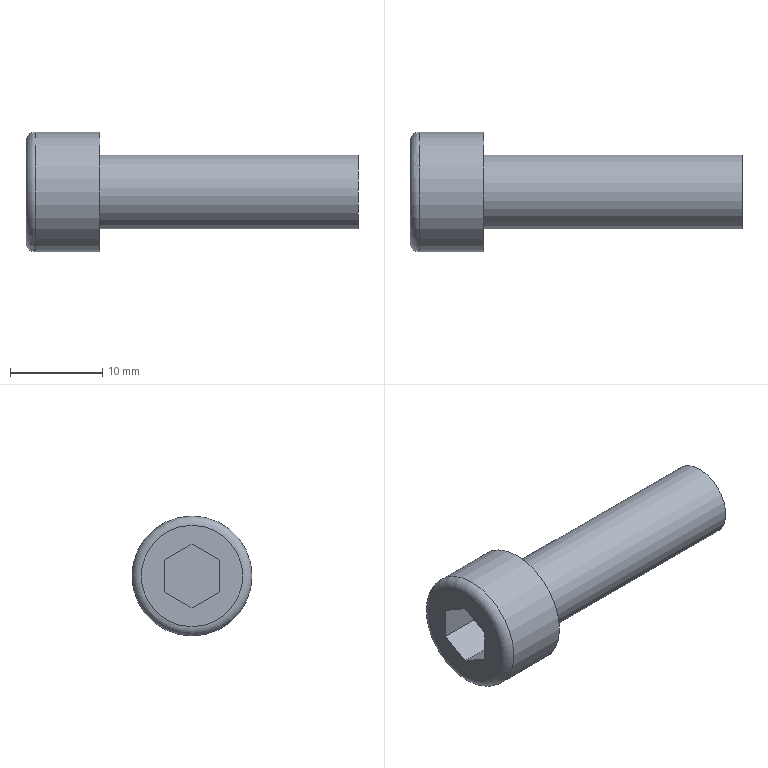Part | STEP file | Tube necking machine_id606_x_t | 1 solid | 13 faces | box 36 x 13 x 13 mm | volume 2296 mm3 | plane 10 | cylinder 2 | torus 1 | commonest cylinder face diameters 8 x1 13 x1
STEP:
#1=CARTESIAN_POINT('',(0.,0.,0.));
#2=DIRECTION('',(0.,0.,1.));
#3=DIRECTION('',(1.,0.,0.));
#4=AXIS2_PLACEMENT_3D('',#1,#2,#3);
#5=CARTESIAN_POINT('',(367.5,70.,164.5));
#6=VERTEX_POINT('',#5);
#7=CARTESIAN_POINT('',(367.5,70.,170.));
#8=DIRECTION('',(-1.,0.,0.));
#9=DIRECTION('',(0.,0.,-1.));
#10=AXIS2_PLACEMENT_3D('',#7,#8,#9);
#11=CIRCLE('',#10,5.5);
#12=CARTESIAN_POINT('',(367.5,70.,176.5));
#13=DIRECTION('',(1.,0.,0.));
#14=DIRECTION('',(0.,0.,-1.));
#15=AXIS2_PLACEMENT_3D('',#12,#13,#14);
#16=PLANE('',#15);
#17=CARTESIAN_POINT('',(12.,0.));
#18=CARTESIAN_POINT('',(12.,-9.526));
#19=CARTESIAN_POINT('',(3.75,-4.763));
#20=CARTESIAN_POINT('',(-4.5,0.));
#21=CARTESIAN_POINT('',(3.75,4.763));
#22=CARTESIAN_POINT('',(12.,9.526));
#23=CARTESIAN_POINT('',(12.,0.));
#24=(BOUNDED_CURVE()B_SPLINE_CURVE(2,(#17,#18,#19,#20,#21,#22,#23),.UNSPECIFIED.,.T.,.F.)B_SPLINE_CURVE_WITH_KNOTS((1,2,2,2,2,1),(-2.094,0.,2.094,4.189,6.283,8.378),.UNSPECIFIED.)CURVE()GEOMETRIC_REPRESENTATION_ITEM()RATIONAL_B_SPLINE_CURVE((1.,0.5,1.,0.5,1.,0.5,1.))REPRESENTATION_ITEM(''));
#25=(GEOMETRIC_REPRESENTATION_CONTEXT(2)PARAMETRIC_REPRESENTATION_CONTEXT()REPRESENTATION_CONTEXT('',''));
#26=DEFINITIONAL_REPRESENTATION('',(#24),#25);
#27=PCURVE('',#16,#26);
#28=CARTESIAN_POINT('',(368.5,70.,170.));
#29=DIRECTION('',(1.,0.,0.));
#30=DIRECTION('',(0.,0.,-1.));
#31=AXIS2_PLACEMENT_3D('',#28,#29,#30);
#32=TOROIDAL_SURFACE('',#31,5.5,1.);
#33=CARTESIAN_POINT('',(6.283,4.712));
#34=DIRECTION('',(-1.,0.));
#35=VECTOR('',#34,1.);
#36=LINE('',#33,#35);
#37=(GEOMETRIC_REPRESENTATION_CONTEXT(2)PARAMETRIC_REPRESENTATION_CONTEXT()REPRESENTATION_CONTEXT('',''));
#38=DEFINITIONAL_REPRESENTATION('',(#36),#37);
#39=PCURVE('',#32,#38);
#40=SURFACE_CURVE('',#11,(#27,#39),.PCURVE_S1.);
#41=EDGE_CURVE('',#6,#6,#40,.T.);
#42=ORIENTED_EDGE('',*,*,#41,.T.);
#43=EDGE_LOOP('',(#42));
#44=FACE_BOUND('',#43,.T.);
#45=CARTESIAN_POINT('',(367.5,73.,168.268));
#46=VERTEX_POINT('',#45);
#47=CARTESIAN_POINT('',(367.5,73.,171.732));
#48=VERTEX_POINT('',#47);
#49=CARTESIAN_POINT('',(367.5,73.,168.268));
#50=DIRECTION('',(0.,0.,1.));
#51=VECTOR('',#50,1.);
#52=LINE('',#49,#51);
#53=CARTESIAN_POINT('',(8.232,3.));
#54=DIRECTION('',(-1.,0.));
#55=VECTOR('',#54,1.);
#56=LINE('',#53,#55);
#57=(GEOMETRIC_REPRESENTATION_CONTEXT(2)PARAMETRIC_REPRESENTATION_CONTEXT()REPRESENTATION_CONTEXT('',''));
#58=DEFINITIONAL_REPRESENTATION('',(#56),#57);
#59=PCURVE('',#16,#58);
#60=CARTESIAN_POINT('',(372.78,73.,168.268));
#61=DIRECTION('',(0.,-1.,0.));
#62=DIRECTION('',(0.,0.,1.));
#63=AXIS2_PLACEMENT_3D('',#60,#61,#62);
#64=PLANE('',#63);
#65=CARTESIAN_POINT('',(0.,5.28));
#66=DIRECTION('',(1.,0.));
#67=VECTOR('',#66,1.);
#68=LINE('',#65,#67);
#69=(GEOMETRIC_REPRESENTATION_CONTEXT(2)PARAMETRIC_REPRESENTATION_CONTEXT()REPRESENTATION_CONTEXT('',''));
#70=DEFINITIONAL_REPRESENTATION('',(#68),#69);
#71=PCURVE('',#64,#70);
#72=SURFACE_CURVE('',#52,(#59,#71),.PCURVE_S1.);
#73=EDGE_CURVE('',#46,#48,#72,.T.);
#74=ORIENTED_EDGE('',*,*,#73,.T.);
#75=CARTESIAN_POINT('',(367.5,70.,173.464));
#76=VERTEX_POINT('',#75);
#77=CARTESIAN_POINT('',(367.5,73.,171.732));
#78=DIRECTION('',(0.,-0.866,0.5));
#79=VECTOR('',#78,1.);
#80=LINE('',#77,#79);
#81=CARTESIAN_POINT('',(4.768,3.));
#82=DIRECTION('',(-0.5,-0.866));
#83=VECTOR('',#82,1.);
#84=LINE('',#81,#83);
#85=(GEOMETRIC_REPRESENTATION_CONTEXT(2)PARAMETRIC_REPRESENTATION_CONTEXT()REPRESENTATION_CONTEXT('',''));
#86=DEFINITIONAL_REPRESENTATION('',(#84),#85);
#87=PCURVE('',#16,#86);
#88=CARTESIAN_POINT('',(372.78,73.,171.732));
#89=DIRECTION('',(0.,-0.5,-0.866));
#90=DIRECTION('',(0.,-0.866,0.5));
#91=AXIS2_PLACEMENT_3D('',#88,#89,#90);
#92=PLANE('',#91);
#93=CARTESIAN_POINT('',(0.,5.28));
#94=DIRECTION('',(1.,0.));
#95=VECTOR('',#94,1.);
#96=LINE('',#93,#95);
#97=(GEOMETRIC_REPRESENTATION_CONTEXT(2)PARAMETRIC_REPRESENTATION_CONTEXT()REPRESENTATION_CONTEXT('',''));
#98=DEFINITIONAL_REPRESENTATION('',(#96),#97);
#99=PCURVE('',#92,#98);
#100=SURFACE_CURVE('',#80,(#87,#99),.PCURVE_S1.);
#101=EDGE_CURVE('',#48,#76,#100,.T.);
#102=ORIENTED_EDGE('',*,*,#101,.T.);
#103=CARTESIAN_POINT('',(367.5,67.,171.732));
#104=VERTEX_POINT('',#103);
#105=CARTESIAN_POINT('',(367.5,70.,173.464));
#106=DIRECTION('',(0.,-0.866,-0.5));
#107=VECTOR('',#106,1.);
#108=LINE('',#105,#107);
#109=CARTESIAN_POINT('',(3.036,0.));
#110=DIRECTION('',(0.5,-0.866));
#111=VECTOR('',#110,1.);
#112=LINE('',#109,#111);
#113=(GEOMETRIC_REPRESENTATION_CONTEXT(2)PARAMETRIC_REPRESENTATION_CONTEXT()REPRESENTATION_CONTEXT('',''));
#114=DEFINITIONAL_REPRESENTATION('',(#112),#113);
#115=PCURVE('',#16,#114);
#116=CARTESIAN_POINT('',(372.78,70.,173.464));
#117=DIRECTION('',(0.,0.5,-0.866));
#118=DIRECTION('',(0.,-0.866,-0.5));
#119=AXIS2_PLACEMENT_3D('',#116,#117,#118);
#120=PLANE('',#119);
#121=CARTESIAN_POINT('',(0.,5.28));
#122=DIRECTION('',(1.,0.));
#123=VECTOR('',#122,1.);
#124=LINE('',#121,#123);
#125=(GEOMETRIC_REPRESENTATION_CONTEXT(2)PARAMETRIC_REPRESENTATION_CONTEXT()REPRESENTATION_CONTEXT('',''));
#126=DEFINITIONAL_REPRESENTATION('',(#124),#125);
#127=PCURVE('',#120,#126);
#128=SURFACE_CURVE('',#108,(#115,#127),.PCURVE_S1.);
#129=EDGE_CURVE('',#76,#104,#128,.T.);
#130=ORIENTED_EDGE('',*,*,#129,.T.);
#131=CARTESIAN_POINT('',(367.5,67.,168.268));
#132=VERTEX_POINT('',#131);
#133=CARTESIAN_POINT('',(367.5,67.,171.732));
#134=DIRECTION('',(0.,0.,-1.));
#135=VECTOR('',#134,1.);
#136=LINE('',#133,#135);
#137=CARTESIAN_POINT('',(4.768,-3.));
#138=DIRECTION('',(1.,0.));
#139=VECTOR('',#138,1.);
#140=LINE('',#137,#139);
#141=(GEOMETRIC_REPRESENTATION_CONTEXT(2)PARAMETRIC_REPRESENTATION_CONTEXT()REPRESENTATION_CONTEXT('',''));
#142=DEFINITIONAL_REPRESENTATION('',(#140),#141);
#143=PCURVE('',#16,#142);
#144=CARTESIAN_POINT('',(372.78,67.,171.732));
#145=DIRECTION('',(0.,1.,0.));
#146=DIRECTION('',(0.,0.,-1.));
#147=AXIS2_PLACEMENT_3D('',#144,#145,#146);
#148=PLANE('',#147);
#149=CARTESIAN_POINT('',(0.,5.28));
#150=DIRECTION('',(1.,0.));
#151=VECTOR('',#150,1.);
#152=LINE('',#149,#151);
#153=(GEOMETRIC_REPRESENTATION_CONTEXT(2)PARAMETRIC_REPRESENTATION_CONTEXT()REPRESENTATION_CONTEXT('',''));
#154=DEFINITIONAL_REPRESENTATION('',(#152),#153);
#155=PCURVE('',#148,#154);
#156=SURFACE_CURVE('',#136,(#143,#155),.PCURVE_S1.);
#157=EDGE_CURVE('',#104,#132,#156,.T.);
#158=ORIENTED_EDGE('',*,*,#157,.T.);
#159=CARTESIAN_POINT('',(367.5,70.,166.536));
#160=VERTEX_POINT('',#159);
#161=CARTESIAN_POINT('',(367.5,67.,168.268));
#162=DIRECTION('',(0.,0.866,-0.5));
#163=VECTOR('',#162,1.);
#164=LINE('',#161,#163);
#165=CARTESIAN_POINT('',(8.232,-3.));
#166=DIRECTION('',(0.5,0.866));
#167=VECTOR('',#166,1.);
#168=LINE('',#165,#167);
#169=(GEOMETRIC_REPRESENTATION_CONTEXT(2)PARAMETRIC_REPRESENTATION_CONTEXT()REPRESENTATION_CONTEXT('',''));
#170=DEFINITIONAL_REPRESENTATION('',(#168),#169);
#171=PCURVE('',#16,#170);
#172=CARTESIAN_POINT('',(372.78,67.,168.268));
#173=DIRECTION('',(0.,0.5,0.866));
#174=DIRECTION('',(0.,0.866,-0.5));
#175=AXIS2_PLACEMENT_3D('',#172,#173,#174);
#176=PLANE('',#175);
#177=CARTESIAN_POINT('',(0.,5.28));
#178=DIRECTION('',(1.,0.));
#179=VECTOR('',#178,1.);
#180=LINE('',#177,#179);
#181=(GEOMETRIC_REPRESENTATION_CONTEXT(2)PARAMETRIC_REPRESENTATION_CONTEXT()REPRESENTATION_CONTEXT('',''));
#182=DEFINITIONAL_REPRESENTATION('',(#180),#181);
#183=PCURVE('',#176,#182);
#184=SURFACE_CURVE('',#164,(#171,#183),.PCURVE_S1.);
#185=EDGE_CURVE('',#132,#160,#184,.T.);
#186=ORIENTED_EDGE('',*,*,#185,.T.);
#187=CARTESIAN_POINT('',(367.5,70.,166.536));
#188=DIRECTION('',(0.,0.866,0.5));
#189=VECTOR('',#188,1.);
#190=LINE('',#187,#189);
#191=CARTESIAN_POINT('',(9.964,0.));
#192=DIRECTION('',(-0.5,0.866));
#193=VECTOR('',#192,1.);
#194=LINE('',#191,#193);
#195=(GEOMETRIC_REPRESENTATION_CONTEXT(2)PARAMETRIC_REPRESENTATION_CONTEXT()REPRESENTATION_CONTEXT('',''));
#196=DEFINITIONAL_REPRESENTATION('',(#194),#195);
#197=PCURVE('',#16,#196);
#198=CARTESIAN_POINT('',(372.78,70.,166.536));
#199=DIRECTION('',(0.,-0.5,0.866));
#200=DIRECTION('',(0.,0.866,0.5));
#201=AXIS2_PLACEMENT_3D('',#198,#199,#200);
#202=PLANE('',#201);
#203=CARTESIAN_POINT('',(0.,5.28));
#204=DIRECTION('',(1.,0.));
#205=VECTOR('',#204,1.);
#206=LINE('',#203,#205);
#207=(GEOMETRIC_REPRESENTATION_CONTEXT(2)PARAMETRIC_REPRESENTATION_CONTEXT()REPRESENTATION_CONTEXT('',''));
#208=DEFINITIONAL_REPRESENTATION('',(#206),#207);
#209=PCURVE('',#202,#208);
#210=SURFACE_CURVE('',#190,(#197,#209),.PCURVE_S1.);
#211=EDGE_CURVE('',#160,#46,#210,.T.);
#212=ORIENTED_EDGE('',*,*,#211,.T.);
#213=EDGE_LOOP('',(#74,#102,#130,#158,#186,#212));
#214=FACE_BOUND('',#213,.T.);
#215=ADVANCED_FACE('',(#44,#214),#16,.F.);
#216=CARTESIAN_POINT('',(368.5,70.,163.5));
#217=VERTEX_POINT('',#216);
#218=CARTESIAN_POINT('',(368.5,70.,176.5));
#219=VERTEX_POINT('',#218);
#220=CARTESIAN_POINT('',(368.5,70.,170.));
#221=DIRECTION('',(1.,0.,0.));
#222=DIRECTION('',(0.,0.,-1.));
#223=AXIS2_PLACEMENT_3D('',#220,#221,#222);
#224=CIRCLE('',#223,6.5);
#225=CARTESIAN_POINT('',(374.4,70.,170.));
#226=DIRECTION('',(-1.,0.,0.));
#227=DIRECTION('',(0.,0.,1.));
#228=AXIS2_PLACEMENT_3D('',#225,#226,#227);
#229=CYLINDRICAL_SURFACE('',#228,6.5);
#230=CARTESIAN_POINT('',(3.142,5.9));
#231=DIRECTION('',(-1.,0.));
#232=VECTOR('',#231,1.);
#233=LINE('',#230,#232);
#234=(GEOMETRIC_REPRESENTATION_CONTEXT(2)PARAMETRIC_REPRESENTATION_CONTEXT()REPRESENTATION_CONTEXT('',''));
#235=DEFINITIONAL_REPRESENTATION('',(#233),#234);
#236=PCURVE('',#229,#235);
#237=CARTESIAN_POINT('',(0.,6.283));
#238=DIRECTION('',(1.,0.));
#239=VECTOR('',#238,1.);
#240=LINE('',#237,#239);
#241=(GEOMETRIC_REPRESENTATION_CONTEXT(2)PARAMETRIC_REPRESENTATION_CONTEXT()REPRESENTATION_CONTEXT('',''));
#242=DEFINITIONAL_REPRESENTATION('',(#240),#241);
#243=PCURVE('',#32,#242);
#244=SURFACE_CURVE('',#224,(#236,#243),.PCURVE_S1.);
#245=EDGE_CURVE('',#217,#219,#244,.T.);
#246=ORIENTED_EDGE('',*,*,#245,.T.);
#247=CARTESIAN_POINT('',(375.5,70.,176.5));
#248=VERTEX_POINT('',#247);
#249=CARTESIAN_POINT('',(375.5,70.,176.5));
#250=CARTESIAN_POINT('',(368.5,70.,176.5));
#251=B_SPLINE_CURVE_WITH_KNOTS('',1,(#249,#250),.UNSPECIFIED.,.F.,.F.,(2,2),(-1.1,5.9),.PIECEWISE_BEZIER_KNOTS.);
#252=CARTESIAN_POINT('',(0.,0.));
#253=DIRECTION('',(0.,1.));
#254=VECTOR('',#253,1.);
#255=LINE('',#252,#254);
#256=(GEOMETRIC_REPRESENTATION_CONTEXT(2)PARAMETRIC_REPRESENTATION_CONTEXT()REPRESENTATION_CONTEXT('',''));
#257=DEFINITIONAL_REPRESENTATION('',(#255),#256);
#258=PCURVE('',#229,#257);
#259=CARTESIAN_POINT('',(6.283,0.));
#260=DIRECTION('',(0.,1.));
#261=VECTOR('',#260,1.);
#262=LINE('',#259,#261);
#263=(GEOMETRIC_REPRESENTATION_CONTEXT(2)PARAMETRIC_REPRESENTATION_CONTEXT()REPRESENTATION_CONTEXT('',''));
#264=DEFINITIONAL_REPRESENTATION('',(#262),#263);
#265=PCURVE('',#229,#264);
#266=SEAM_CURVE('',#251,(#258,#265),.PCURVE_S1.);
#267=EDGE_CURVE('',#248,#219,#266,.T.);
#268=ORIENTED_EDGE('',*,*,#267,.F.);
#269=CARTESIAN_POINT('',(375.5,70.,170.));
#270=DIRECTION('',(-1.,0.,0.));
#271=DIRECTION('',(0.,0.,1.));
#272=AXIS2_PLACEMENT_3D('',#269,#270,#271);
#273=CIRCLE('',#272,6.5);
#274=CARTESIAN_POINT('',(0.,-1.1));
#275=DIRECTION('',(1.,0.));
#276=VECTOR('',#275,1.);
#277=LINE('',#274,#276);
#278=(GEOMETRIC_REPRESENTATION_CONTEXT(2)PARAMETRIC_REPRESENTATION_CONTEXT()REPRESENTATION_CONTEXT('',''));
#279=DEFINITIONAL_REPRESENTATION('',(#277),#278);
#280=PCURVE('',#229,#279);
#281=CARTESIAN_POINT('',(375.5,70.,174.));
#282=DIRECTION('',(-1.,0.,0.));
#283=DIRECTION('',(0.,0.,1.));
#284=AXIS2_PLACEMENT_3D('',#281,#282,#283);
#285=PLANE('',#284);
#286=CARTESIAN_POINT('',(-4.,0.));
#287=DIRECTION('',(1.,0.));
#288=AXIS2_PLACEMENT_2D('',#286,#287);
#289=CIRCLE('',#288,6.5);
#290=(GEOMETRIC_REPRESENTATION_CONTEXT(2)PARAMETRIC_REPRESENTATION_CONTEXT()REPRESENTATION_CONTEXT('',''));
#291=DEFINITIONAL_REPRESENTATION('',(#289),#290);
#292=PCURVE('',#285,#291);
#293=SURFACE_CURVE('',#273,(#280,#292),.PCURVE_S1.);
#294=EDGE_CURVE('',#248,#248,#293,.T.);
#295=ORIENTED_EDGE('',*,*,#294,.T.);
#296=ORIENTED_EDGE('',*,*,#267,.T.);
#297=CARTESIAN_POINT('',(368.5,70.,170.));
#298=DIRECTION('',(1.,0.,0.));
#299=DIRECTION('',(0.,0.,-1.));
#300=AXIS2_PLACEMENT_3D('',#297,#298,#299);
#301=CIRCLE('',#300,6.5);
#302=CARTESIAN_POINT('',(9.425,5.9));
#303=DIRECTION('',(-1.,0.));
#304=VECTOR('',#303,1.);
#305=LINE('',#302,#304);
#306=(GEOMETRIC_REPRESENTATION_CONTEXT(2)PARAMETRIC_REPRESENTATION_CONTEXT()REPRESENTATION_CONTEXT('',''));
#307=DEFINITIONAL_REPRESENTATION('',(#305),#306);
#308=PCURVE('',#229,#307);
#309=CARTESIAN_POINT('',(0.,6.283));
#310=DIRECTION('',(1.,0.));
#311=VECTOR('',#310,1.);
#312=LINE('',#309,#311);
#313=(GEOMETRIC_REPRESENTATION_CONTEXT(2)PARAMETRIC_REPRESENTATION_CONTEXT()REPRESENTATION_CONTEXT('',''));
#314=DEFINITIONAL_REPRESENTATION('',(#312),#313);
#315=PCURVE('',#32,#314);
#316=SURFACE_CURVE('',#301,(#308,#315),.PCURVE_S1.);
#317=EDGE_CURVE('',#219,#217,#316,.T.);
#318=ORIENTED_EDGE('',*,*,#317,.T.);
#319=EDGE_LOOP('',(#246,#268,#295,#296,#318));
#320=FACE_BOUND('',#319,.T.);
#321=ADVANCED_FACE('',(#320),#229,.T.);
#322=ORIENTED_EDGE('',*,*,#294,.F.);
#323=EDGE_LOOP('',(#322));
#324=FACE_BOUND('',#323,.T.);
#325=CARTESIAN_POINT('',(375.5,70.,174.));
#326=VERTEX_POINT('',#325);
#327=CARTESIAN_POINT('',(375.5,70.,170.));
#328=DIRECTION('',(-1.,0.,0.));
#329=DIRECTION('',(0.,0.,1.));
#330=AXIS2_PLACEMENT_3D('',#327,#328,#329);
#331=CIRCLE('',#330,4.);
#332=CARTESIAN_POINT('',(-4.,0.));
#333=DIRECTION('',(1.,0.));
#334=AXIS2_PLACEMENT_2D('',#332,#333);
#335=CIRCLE('',#334,4.);
#336=(GEOMETRIC_REPRESENTATION_CONTEXT(2)PARAMETRIC_REPRESENTATION_CONTEXT()REPRESENTATION_CONTEXT('',''));
#337=DEFINITIONAL_REPRESENTATION('',(#335),#336);
#338=PCURVE('',#285,#337);
#339=CARTESIAN_POINT('',(374.4,70.,170.));
#340=DIRECTION('',(-1.,0.,0.));
#341=DIRECTION('',(0.,0.,1.));
#342=AXIS2_PLACEMENT_3D('',#339,#340,#341);
#343=CYLINDRICAL_SURFACE('',#342,4.);
#344=CARTESIAN_POINT('',(0.,-1.1));
#345=DIRECTION('',(1.,0.));
#346=VECTOR('',#345,1.);
#347=LINE('',#344,#346);
#348=(GEOMETRIC_REPRESENTATION_CONTEXT(2)PARAMETRIC_REPRESENTATION_CONTEXT()REPRESENTATION_CONTEXT('',''));
#349=DEFINITIONAL_REPRESENTATION('',(#347),#348);
#350=PCURVE('',#343,#349);
#351=SURFACE_CURVE('',#331,(#338,#350),.PCURVE_S1.);
#352=EDGE_CURVE('',#326,#326,#351,.T.);
#353=ORIENTED_EDGE('',*,*,#352,.T.);
#354=EDGE_LOOP('',(#353));
#355=FACE_BOUND('',#354,.T.);
#356=ADVANCED_FACE('',(#324,#355),#285,.F.);
#357=ORIENTED_EDGE('',*,*,#352,.F.);
#358=CARTESIAN_POINT('',(403.5,70.,174.));
#359=VERTEX_POINT('',#358);
#360=CARTESIAN_POINT('',(403.5,70.,174.));
#361=CARTESIAN_POINT('',(375.5,70.,174.));
#362=B_SPLINE_CURVE_WITH_KNOTS('',1,(#360,#361),.UNSPECIFIED.,.F.,.F.,(2,2),(-29.1,-1.1),.PIECEWISE_BEZIER_KNOTS.);
#363=CARTESIAN_POINT('',(0.,0.));
#364=DIRECTION('',(0.,1.));
#365=VECTOR('',#364,1.);
#366=LINE('',#363,#365);
#367=(GEOMETRIC_REPRESENTATION_CONTEXT(2)PARAMETRIC_REPRESENTATION_CONTEXT()REPRESENTATION_CONTEXT('',''));
#368=DEFINITIONAL_REPRESENTATION('',(#366),#367);
#369=PCURVE('',#343,#368);
#370=CARTESIAN_POINT('',(6.283,0.));
#371=DIRECTION('',(0.,1.));
#372=VECTOR('',#371,1.);
#373=LINE('',#370,#372);
#374=(GEOMETRIC_REPRESENTATION_CONTEXT(2)PARAMETRIC_REPRESENTATION_CONTEXT()REPRESENTATION_CONTEXT('',''));
#375=DEFINITIONAL_REPRESENTATION('',(#373),#374);
#376=PCURVE('',#343,#375);
#377=SEAM_CURVE('',#362,(#369,#376),.PCURVE_S1.);
#378=EDGE_CURVE('',#359,#326,#377,.T.);
#379=ORIENTED_EDGE('',*,*,#378,.F.);
#380=CARTESIAN_POINT('',(403.5,70.,170.));
#381=DIRECTION('',(-1.,0.,0.));
#382=DIRECTION('',(0.,0.,1.));
#383=AXIS2_PLACEMENT_3D('',#380,#381,#382);
#384=CIRCLE('',#383,4.);
#385=CARTESIAN_POINT('',(0.,-29.1));
#386=DIRECTION('',(1.,0.));
#387=VECTOR('',#386,1.);
#388=LINE('',#385,#387);
#389=(GEOMETRIC_REPRESENTATION_CONTEXT(2)PARAMETRIC_REPRESENTATION_CONTEXT()REPRESENTATION_CONTEXT('',''));
#390=DEFINITIONAL_REPRESENTATION('',(#388),#389);
#391=PCURVE('',#343,#390);
#392=CARTESIAN_POINT('',(403.5,70.,170.));
#393=DIRECTION('',(-1.,0.,0.));
#394=DIRECTION('',(0.,0.,1.));
#395=AXIS2_PLACEMENT_3D('',#392,#393,#394);
#396=PLANE('',#395);
#397=CARTESIAN_POINT('',(0.,0.));
#398=DIRECTION('',(1.,0.));
#399=AXIS2_PLACEMENT_2D('',#397,#398);
#400=CIRCLE('',#399,4.);
#401=(GEOMETRIC_REPRESENTATION_CONTEXT(2)PARAMETRIC_REPRESENTATION_CONTEXT()REPRESENTATION_CONTEXT('',''));
#402=DEFINITIONAL_REPRESENTATION('',(#400),#401);
#403=PCURVE('',#396,#402);
#404=SURFACE_CURVE('',#384,(#391,#403),.PCURVE_S1.);
#405=EDGE_CURVE('',#359,#359,#404,.T.);
#406=ORIENTED_EDGE('',*,*,#405,.T.);
#407=ORIENTED_EDGE('',*,*,#378,.T.);
#408=EDGE_LOOP('',(#357,#379,#406,#407));
#409=FACE_BOUND('',#408,.T.);
#410=ADVANCED_FACE('',(#409),#343,.T.);
#411=ORIENTED_EDGE('',*,*,#405,.F.);
#412=EDGE_LOOP('',(#411));
#413=FACE_BOUND('',#412,.T.);
#414=ADVANCED_FACE('',(#413),#396,.F.);
#415=ORIENTED_EDGE('',*,*,#73,.F.);
#416=CARTESIAN_POINT('',(372.78,73.,168.268));
#417=VERTEX_POINT('',#416);
#418=CARTESIAN_POINT('',(372.78,73.,168.268));
#419=DIRECTION('',(1.,0.,0.));
#420=VECTOR('',#419,1.);
#421=LINE('',#418,#420);
#422=CARTESIAN_POINT('',(0.,0.));
#423=DIRECTION('',(0.,-1.));
#424=VECTOR('',#423,1.);
#425=LINE('',#422,#424);
#426=(GEOMETRIC_REPRESENTATION_CONTEXT(2)PARAMETRIC_REPRESENTATION_CONTEXT()REPRESENTATION_CONTEXT('',''));
#427=DEFINITIONAL_REPRESENTATION('',(#425),#426);
#428=PCURVE('',#64,#427);
#429=CARTESIAN_POINT('',(3.464,0.));
#430=DIRECTION('',(0.,-1.));
#431=VECTOR('',#430,1.);
#432=LINE('',#429,#431);
#433=(GEOMETRIC_REPRESENTATION_CONTEXT(2)PARAMETRIC_REPRESENTATION_CONTEXT()REPRESENTATION_CONTEXT('',''));
#434=DEFINITIONAL_REPRESENTATION('',(#432),#433);
#435=PCURVE('',#202,#434);
#436=SURFACE_CURVE('',#421,(#428,#435),.PCURVE_S1.);
#437=EDGE_CURVE('',#46,#417,#436,.T.);
#438=ORIENTED_EDGE('',*,*,#437,.T.);
#439=CARTESIAN_POINT('',(372.78,73.,171.732));
#440=VERTEX_POINT('',#439);
#441=CARTESIAN_POINT('',(372.78,73.,168.268));
#442=DIRECTION('',(0.,0.,-1.));
#443=VECTOR('',#442,1.);
#444=LINE('',#441,#443);
#445=CARTESIAN_POINT('',(0.,0.));
#446=DIRECTION('',(-1.,0.));
#447=VECTOR('',#446,1.);
#448=LINE('',#445,#447);
#449=(GEOMETRIC_REPRESENTATION_CONTEXT(2)PARAMETRIC_REPRESENTATION_CONTEXT()REPRESENTATION_CONTEXT('',''));
#450=DEFINITIONAL_REPRESENTATION('',(#448),#449);
#451=PCURVE('',#64,#450);
#452=CARTESIAN_POINT('',(372.78,70.,170.));
#453=DIRECTION('',(1.,0.,0.));
#454=DIRECTION('',(0.,0.,-1.));
#455=AXIS2_PLACEMENT_3D('',#452,#453,#454);
#456=PLANE('',#455);
#457=CARTESIAN_POINT('',(1.732,3.));
#458=DIRECTION('',(1.,0.));
#459=VECTOR('',#458,1.);
#460=LINE('',#457,#459);
#461=(GEOMETRIC_REPRESENTATION_CONTEXT(2)PARAMETRIC_REPRESENTATION_CONTEXT()REPRESENTATION_CONTEXT('',''));
#462=DEFINITIONAL_REPRESENTATION('',(#460),#461);
#463=PCURVE('',#456,#462);
#464=SURFACE_CURVE('',#444,(#451,#463),.PCURVE_S1.);
#465=EDGE_CURVE('',#440,#417,#464,.T.);
#466=ORIENTED_EDGE('',*,*,#465,.F.);
#467=CARTESIAN_POINT('',(372.78,73.,171.732));
#468=DIRECTION('',(1.,0.,0.));
#469=VECTOR('',#468,1.);
#470=LINE('',#467,#469);
#471=CARTESIAN_POINT('',(3.464,0.));
#472=DIRECTION('',(0.,-1.));
#473=VECTOR('',#472,1.);
#474=LINE('',#471,#473);
#475=(GEOMETRIC_REPRESENTATION_CONTEXT(2)PARAMETRIC_REPRESENTATION_CONTEXT()REPRESENTATION_CONTEXT('',''));
#476=DEFINITIONAL_REPRESENTATION('',(#474),#475);
#477=PCURVE('',#64,#476);
#478=CARTESIAN_POINT('',(0.,0.));
#479=DIRECTION('',(0.,-1.));
#480=VECTOR('',#479,1.);
#481=LINE('',#478,#480);
#482=(GEOMETRIC_REPRESENTATION_CONTEXT(2)PARAMETRIC_REPRESENTATION_CONTEXT()REPRESENTATION_CONTEXT('',''));
#483=DEFINITIONAL_REPRESENTATION('',(#481),#482);
#484=PCURVE('',#92,#483);
#485=SURFACE_CURVE('',#470,(#477,#484),.PCURVE_S1.);
#486=EDGE_CURVE('',#48,#440,#485,.T.);
#487=ORIENTED_EDGE('',*,*,#486,.F.);
#488=EDGE_LOOP('',(#415,#438,#466,#487));
#489=FACE_BOUND('',#488,.T.);
#490=ADVANCED_FACE('',(#489),#64,.T.);
#491=ORIENTED_EDGE('',*,*,#101,.F.);
#492=ORIENTED_EDGE('',*,*,#486,.T.);
#493=CARTESIAN_POINT('',(372.78,70.,173.464));
#494=VERTEX_POINT('',#493);
#495=CARTESIAN_POINT('',(372.78,73.,171.732));
#496=DIRECTION('',(0.,0.866,-0.5));
#497=VECTOR('',#496,1.);
#498=LINE('',#495,#497);
#499=CARTESIAN_POINT('',(0.,0.));
#500=DIRECTION('',(-1.,0.));
#501=VECTOR('',#500,1.);
#502=LINE('',#499,#501);
#503=(GEOMETRIC_REPRESENTATION_CONTEXT(2)PARAMETRIC_REPRESENTATION_CONTEXT()REPRESENTATION_CONTEXT('',''));
#504=DEFINITIONAL_REPRESENTATION('',(#502),#503);
#505=PCURVE('',#92,#504);
#506=CARTESIAN_POINT('',(-1.732,3.));
#507=DIRECTION('',(0.5,0.866));
#508=VECTOR('',#507,1.);
#509=LINE('',#506,#508);
#510=(GEOMETRIC_REPRESENTATION_CONTEXT(2)PARAMETRIC_REPRESENTATION_CONTEXT()REPRESENTATION_CONTEXT('',''));
#511=DEFINITIONAL_REPRESENTATION('',(#509),#510);
#512=PCURVE('',#456,#511);
#513=SURFACE_CURVE('',#498,(#505,#512),.PCURVE_S1.);
#514=EDGE_CURVE('',#494,#440,#513,.T.);
#515=ORIENTED_EDGE('',*,*,#514,.F.);
#516=CARTESIAN_POINT('',(372.78,70.,173.464));
#517=DIRECTION('',(1.,0.,0.));
#518=VECTOR('',#517,1.);
#519=LINE('',#516,#518);
#520=CARTESIAN_POINT('',(3.464,0.));
#521=DIRECTION('',(0.,-1.));
#522=VECTOR('',#521,1.);
#523=LINE('',#520,#522);
#524=(GEOMETRIC_REPRESENTATION_CONTEXT(2)PARAMETRIC_REPRESENTATION_CONTEXT()REPRESENTATION_CONTEXT('',''));
#525=DEFINITIONAL_REPRESENTATION('',(#523),#524);
#526=PCURVE('',#92,#525);
#527=CARTESIAN_POINT('',(0.,0.));
#528=DIRECTION('',(0.,-1.));
#529=VECTOR('',#528,1.);
#530=LINE('',#527,#529);
#531=(GEOMETRIC_REPRESENTATION_CONTEXT(2)PARAMETRIC_REPRESENTATION_CONTEXT()REPRESENTATION_CONTEXT('',''));
#532=DEFINITIONAL_REPRESENTATION('',(#530),#531);
#533=PCURVE('',#120,#532);
#534=SURFACE_CURVE('',#519,(#526,#533),.PCURVE_S1.);
#535=EDGE_CURVE('',#76,#494,#534,.T.);
#536=ORIENTED_EDGE('',*,*,#535,.F.);
#537=EDGE_LOOP('',(#491,#492,#515,#536));
#538=FACE_BOUND('',#537,.T.);
#539=ADVANCED_FACE('',(#538),#92,.T.);
#540=ORIENTED_EDGE('',*,*,#129,.F.);
#541=ORIENTED_EDGE('',*,*,#535,.T.);
#542=CARTESIAN_POINT('',(372.78,67.,171.732));
#543=VERTEX_POINT('',#542);
#544=CARTESIAN_POINT('',(372.78,70.,173.464));
#545=DIRECTION('',(0.,0.866,0.5));
#546=VECTOR('',#545,1.);
#547=LINE('',#544,#546);
#548=CARTESIAN_POINT('',(0.,0.));
#549=DIRECTION('',(-1.,0.));
#550=VECTOR('',#549,1.);
#551=LINE('',#548,#550);
#552=(GEOMETRIC_REPRESENTATION_CONTEXT(2)PARAMETRIC_REPRESENTATION_CONTEXT()REPRESENTATION_CONTEXT('',''));
#553=DEFINITIONAL_REPRESENTATION('',(#551),#552);
#554=PCURVE('',#120,#553);
#555=CARTESIAN_POINT('',(-3.464,0.));
#556=DIRECTION('',(-0.5,0.866));
#557=VECTOR('',#556,1.);
#558=LINE('',#555,#557);
#559=(GEOMETRIC_REPRESENTATION_CONTEXT(2)PARAMETRIC_REPRESENTATION_CONTEXT()REPRESENTATION_CONTEXT('',''));
#560=DEFINITIONAL_REPRESENTATION('',(#558),#559);
#561=PCURVE('',#456,#560);
#562=SURFACE_CURVE('',#547,(#554,#561),.PCURVE_S1.);
#563=EDGE_CURVE('',#543,#494,#562,.T.);
#564=ORIENTED_EDGE('',*,*,#563,.F.);
#565=CARTESIAN_POINT('',(372.78,67.,171.732));
#566=DIRECTION('',(1.,0.,0.));
#567=VECTOR('',#566,1.);
#568=LINE('',#565,#567);
#569=CARTESIAN_POINT('',(3.464,0.));
#570=DIRECTION('',(0.,-1.));
#571=VECTOR('',#570,1.);
#572=LINE('',#569,#571);
#573=(GEOMETRIC_REPRESENTATION_CONTEXT(2)PARAMETRIC_REPRESENTATION_CONTEXT()REPRESENTATION_CONTEXT('',''));
#574=DEFINITIONAL_REPRESENTATION('',(#572),#573);
#575=PCURVE('',#120,#574);
#576=CARTESIAN_POINT('',(0.,0.));
#577=DIRECTION('',(0.,-1.));
#578=VECTOR('',#577,1.);
#579=LINE('',#576,#578);
#580=(GEOMETRIC_REPRESENTATION_CONTEXT(2)PARAMETRIC_REPRESENTATION_CONTEXT()REPRESENTATION_CONTEXT('',''));
#581=DEFINITIONAL_REPRESENTATION('',(#579),#580);
#582=PCURVE('',#148,#581);
#583=SURFACE_CURVE('',#568,(#575,#582),.PCURVE_S1.);
#584=EDGE_CURVE('',#104,#543,#583,.T.);
#585=ORIENTED_EDGE('',*,*,#584,.F.);
#586=EDGE_LOOP('',(#540,#541,#564,#585));
#587=FACE_BOUND('',#586,.T.);
#588=ADVANCED_FACE('',(#587),#120,.T.);
#589=ORIENTED_EDGE('',*,*,#157,.F.);
#590=ORIENTED_EDGE('',*,*,#584,.T.);
#591=CARTESIAN_POINT('',(372.78,67.,168.268));
#592=VERTEX_POINT('',#591);
#593=CARTESIAN_POINT('',(372.78,67.,171.732));
#594=DIRECTION('',(0.,0.,1.));
#595=VECTOR('',#594,1.);
#596=LINE('',#593,#595);
#597=CARTESIAN_POINT('',(0.,0.));
#598=DIRECTION('',(-1.,0.));
#599=VECTOR('',#598,1.);
#600=LINE('',#597,#599);
#601=(GEOMETRIC_REPRESENTATION_CONTEXT(2)PARAMETRIC_REPRESENTATION_CONTEXT()REPRESENTATION_CONTEXT('',''));
#602=DEFINITIONAL_REPRESENTATION('',(#600),#601);
#603=PCURVE('',#148,#602);
#604=CARTESIAN_POINT('',(-1.732,-3.));
#605=DIRECTION('',(-1.,0.));
#606=VECTOR('',#605,1.);
#607=LINE('',#604,#606);
#608=(GEOMETRIC_REPRESENTATION_CONTEXT(2)PARAMETRIC_REPRESENTATION_CONTEXT()REPRESENTATION_CONTEXT('',''));
#609=DEFINITIONAL_REPRESENTATION('',(#607),#608);
#610=PCURVE('',#456,#609);
#611=SURFACE_CURVE('',#596,(#603,#610),.PCURVE_S1.);
#612=EDGE_CURVE('',#592,#543,#611,.T.);
#613=ORIENTED_EDGE('',*,*,#612,.F.);
#614=CARTESIAN_POINT('',(372.78,67.,168.268));
#615=DIRECTION('',(1.,0.,0.));
#616=VECTOR('',#615,1.);
#617=LINE('',#614,#616);
#618=CARTESIAN_POINT('',(3.464,0.));
#619=DIRECTION('',(0.,-1.));
#620=VECTOR('',#619,1.);
#621=LINE('',#618,#620);
#622=(GEOMETRIC_REPRESENTATION_CONTEXT(2)PARAMETRIC_REPRESENTATION_CONTEXT()REPRESENTATION_CONTEXT('',''));
#623=DEFINITIONAL_REPRESENTATION('',(#621),#622);
#624=PCURVE('',#148,#623);
#625=CARTESIAN_POINT('',(0.,0.));
#626=DIRECTION('',(0.,-1.));
#627=VECTOR('',#626,1.);
#628=LINE('',#625,#627);
#629=(GEOMETRIC_REPRESENTATION_CONTEXT(2)PARAMETRIC_REPRESENTATION_CONTEXT()REPRESENTATION_CONTEXT('',''));
#630=DEFINITIONAL_REPRESENTATION('',(#628),#629);
#631=PCURVE('',#176,#630);
#632=SURFACE_CURVE('',#617,(#624,#631),.PCURVE_S1.);
#633=EDGE_CURVE('',#132,#592,#632,.T.);
#634=ORIENTED_EDGE('',*,*,#633,.F.);
#635=EDGE_LOOP('',(#589,#590,#613,#634));
#636=FACE_BOUND('',#635,.T.);
#637=ADVANCED_FACE('',(#636),#148,.T.);
#638=ORIENTED_EDGE('',*,*,#185,.F.);
#639=ORIENTED_EDGE('',*,*,#633,.T.);
#640=CARTESIAN_POINT('',(372.78,70.,166.536));
#641=VERTEX_POINT('',#640);
#642=CARTESIAN_POINT('',(372.78,67.,168.268));
#643=DIRECTION('',(0.,-0.866,0.5));
#644=VECTOR('',#643,1.);
#645=LINE('',#642,#644);
#646=CARTESIAN_POINT('',(0.,0.));
#647=DIRECTION('',(-1.,0.));
#648=VECTOR('',#647,1.);
#649=LINE('',#646,#648);
#650=(GEOMETRIC_REPRESENTATION_CONTEXT(2)PARAMETRIC_REPRESENTATION_CONTEXT()REPRESENTATION_CONTEXT('',''));
#651=DEFINITIONAL_REPRESENTATION('',(#649),#650);
#652=PCURVE('',#176,#651);
#653=CARTESIAN_POINT('',(1.732,-3.));
#654=DIRECTION('',(-0.5,-0.866));
#655=VECTOR('',#654,1.);
#656=LINE('',#653,#655);
#657=(GEOMETRIC_REPRESENTATION_CONTEXT(2)PARAMETRIC_REPRESENTATION_CONTEXT()REPRESENTATION_CONTEXT('',''));
#658=DEFINITIONAL_REPRESENTATION('',(#656),#657);
#659=PCURVE('',#456,#658);
#660=SURFACE_CURVE('',#645,(#652,#659),.PCURVE_S1.);
#661=EDGE_CURVE('',#641,#592,#660,.T.);
#662=ORIENTED_EDGE('',*,*,#661,.F.);
#663=CARTESIAN_POINT('',(372.78,70.,166.536));
#664=DIRECTION('',(1.,0.,0.));
#665=VECTOR('',#664,1.);
#666=LINE('',#663,#665);
#667=CARTESIAN_POINT('',(3.464,0.));
#668=DIRECTION('',(0.,-1.));
#669=VECTOR('',#668,1.);
#670=LINE('',#667,#669);
#671=(GEOMETRIC_REPRESENTATION_CONTEXT(2)PARAMETRIC_REPRESENTATION_CONTEXT()REPRESENTATION_CONTEXT('',''));
#672=DEFINITIONAL_REPRESENTATION('',(#670),#671);
#673=PCURVE('',#176,#672);
#674=CARTESIAN_POINT('',(0.,0.));
#675=DIRECTION('',(0.,-1.));
#676=VECTOR('',#675,1.);
#677=LINE('',#674,#676);
#678=(GEOMETRIC_REPRESENTATION_CONTEXT(2)PARAMETRIC_REPRESENTATION_CONTEXT()REPRESENTATION_CONTEXT('',''));
#679=DEFINITIONAL_REPRESENTATION('',(#677),#678);
#680=PCURVE('',#202,#679);
#681=SURFACE_CURVE('',#666,(#673,#680),.PCURVE_S1.);
#682=EDGE_CURVE('',#160,#641,#681,.T.);
#683=ORIENTED_EDGE('',*,*,#682,.F.);
#684=EDGE_LOOP('',(#638,#639,#662,#683));
#685=FACE_BOUND('',#684,.T.);
#686=ADVANCED_FACE('',(#685),#176,.T.);
#687=ORIENTED_EDGE('',*,*,#211,.F.);
#688=ORIENTED_EDGE('',*,*,#682,.T.);
#689=CARTESIAN_POINT('',(372.78,70.,166.536));
#690=DIRECTION('',(0.,-0.866,-0.5));
#691=VECTOR('',#690,1.);
#692=LINE('',#689,#691);
#693=CARTESIAN_POINT('',(0.,0.));
#694=DIRECTION('',(-1.,0.));
#695=VECTOR('',#694,1.);
#696=LINE('',#693,#695);
#697=(GEOMETRIC_REPRESENTATION_CONTEXT(2)PARAMETRIC_REPRESENTATION_CONTEXT()REPRESENTATION_CONTEXT('',''));
#698=DEFINITIONAL_REPRESENTATION('',(#696),#697);
#699=PCURVE('',#202,#698);
#700=CARTESIAN_POINT('',(3.464,0.));
#701=DIRECTION('',(0.5,-0.866));
#702=VECTOR('',#701,1.);
#703=LINE('',#700,#702);
#704=(GEOMETRIC_REPRESENTATION_CONTEXT(2)PARAMETRIC_REPRESENTATION_CONTEXT()REPRESENTATION_CONTEXT('',''));
#705=DEFINITIONAL_REPRESENTATION('',(#703),#704);
#706=PCURVE('',#456,#705);
#707=SURFACE_CURVE('',#692,(#699,#706),.PCURVE_S1.);
#708=EDGE_CURVE('',#417,#641,#707,.T.);
#709=ORIENTED_EDGE('',*,*,#708,.F.);
#710=ORIENTED_EDGE('',*,*,#437,.F.);
#711=EDGE_LOOP('',(#687,#688,#709,#710));
#712=FACE_BOUND('',#711,.T.);
#713=ADVANCED_FACE('',(#712),#202,.T.);
#714=ORIENTED_EDGE('',*,*,#465,.T.);
#715=ORIENTED_EDGE('',*,*,#708,.T.);
#716=ORIENTED_EDGE('',*,*,#661,.T.);
#717=ORIENTED_EDGE('',*,*,#612,.T.);
#718=ORIENTED_EDGE('',*,*,#563,.T.);
#719=ORIENTED_EDGE('',*,*,#514,.T.);
#720=EDGE_LOOP('',(#714,#715,#716,#717,#718,#719));
#721=FACE_BOUND('',#720,.T.);
#722=ADVANCED_FACE('',(#721),#456,.F.);
#723=ORIENTED_EDGE('',*,*,#245,.F.);
#724=CARTESIAN_POINT('',(367.5,70.,164.5));
#725=CARTESIAN_POINT('',(367.5,70.,164.233));
#726=CARTESIAN_POINT('',(367.585,70.,163.972));
#727=CARTESIAN_POINT('',(367.748,70.,163.748));
#728=CARTESIAN_POINT('',(367.972,70.,163.585));
#729=CARTESIAN_POINT('',(368.233,70.,163.5));
#730=CARTESIAN_POINT('',(368.5,70.,163.5));
#731=(BOUNDED_CURVE()B_SPLINE_CURVE(6,(#724,#725,#726,#727,#728,#729,#730),.UNSPECIFIED.,.F.,.F.)B_SPLINE_CURVE_WITH_KNOTS((7,7),(-1.571,0.),.PIECEWISE_BEZIER_KNOTS.)CURVE()GEOMETRIC_REPRESENTATION_ITEM()RATIONAL_B_SPLINE_CURVE((1.031,1.01,0.9979,0.994,0.9979,1.01,1.031))REPRESENTATION_ITEM(''));
#732=CARTESIAN_POINT('',(0.,6.283));
#733=DIRECTION('',(0.,1.));
#734=VECTOR('',#733,1.);
#735=LINE('',#732,#734);
#736=(GEOMETRIC_REPRESENTATION_CONTEXT(2)PARAMETRIC_REPRESENTATION_CONTEXT()REPRESENTATION_CONTEXT('',''));
#737=DEFINITIONAL_REPRESENTATION('',(#735),#736);
#738=PCURVE('',#32,#737);
#739=CARTESIAN_POINT('',(6.283,6.283));
#740=DIRECTION('',(0.,1.));
#741=VECTOR('',#740,1.);
#742=LINE('',#739,#741);
#743=(GEOMETRIC_REPRESENTATION_CONTEXT(2)PARAMETRIC_REPRESENTATION_CONTEXT()REPRESENTATION_CONTEXT('',''));
#744=DEFINITIONAL_REPRESENTATION('',(#742),#743);
#745=PCURVE('',#32,#744);
#746=SEAM_CURVE('',#731,(#738,#745),.PCURVE_S1.);
#747=EDGE_CURVE('',#6,#217,#746,.T.);
#748=ORIENTED_EDGE('',*,*,#747,.F.);
#749=ORIENTED_EDGE('',*,*,#41,.F.);
#750=ORIENTED_EDGE('',*,*,#747,.T.);
#751=ORIENTED_EDGE('',*,*,#317,.F.);
#752=EDGE_LOOP('',(#723,#748,#749,#750,#751));
#753=FACE_BOUND('',#752,.T.);
#754=ADVANCED_FACE('',(#753),#32,.T.);
#755=CLOSED_SHELL('',(#215,#321,#356,#410,#414,#490,#539,#588,#637,#686,#713,#722,#754));
#756=MANIFOLD_SOLID_BREP('',#755);
#757=(LENGTH_UNIT()NAMED_UNIT(*)SI_UNIT(.MILLI.,.METRE.));
#758=UNCERTAINTY_MEASURE_WITH_UNIT(LENGTH_MEASURE(0.000002),#757,'','');
#759=(NAMED_UNIT(*)PLANE_ANGLE_UNIT()SI_UNIT($,.RADIAN.));
#760=(NAMED_UNIT(*)SI_UNIT($,.STERADIAN.)SOLID_ANGLE_UNIT());
#761=(GEOMETRIC_REPRESENTATION_CONTEXT(3)GLOBAL_UNCERTAINTY_ASSIGNED_CONTEXT((#758))GLOBAL_UNIT_ASSIGNED_CONTEXT((#757,#759,#760))REPRESENTATION_CONTEXT('',''));
#762=ADVANCED_BREP_SHAPE_REPRESENTATION('',(#4,#756),#761);